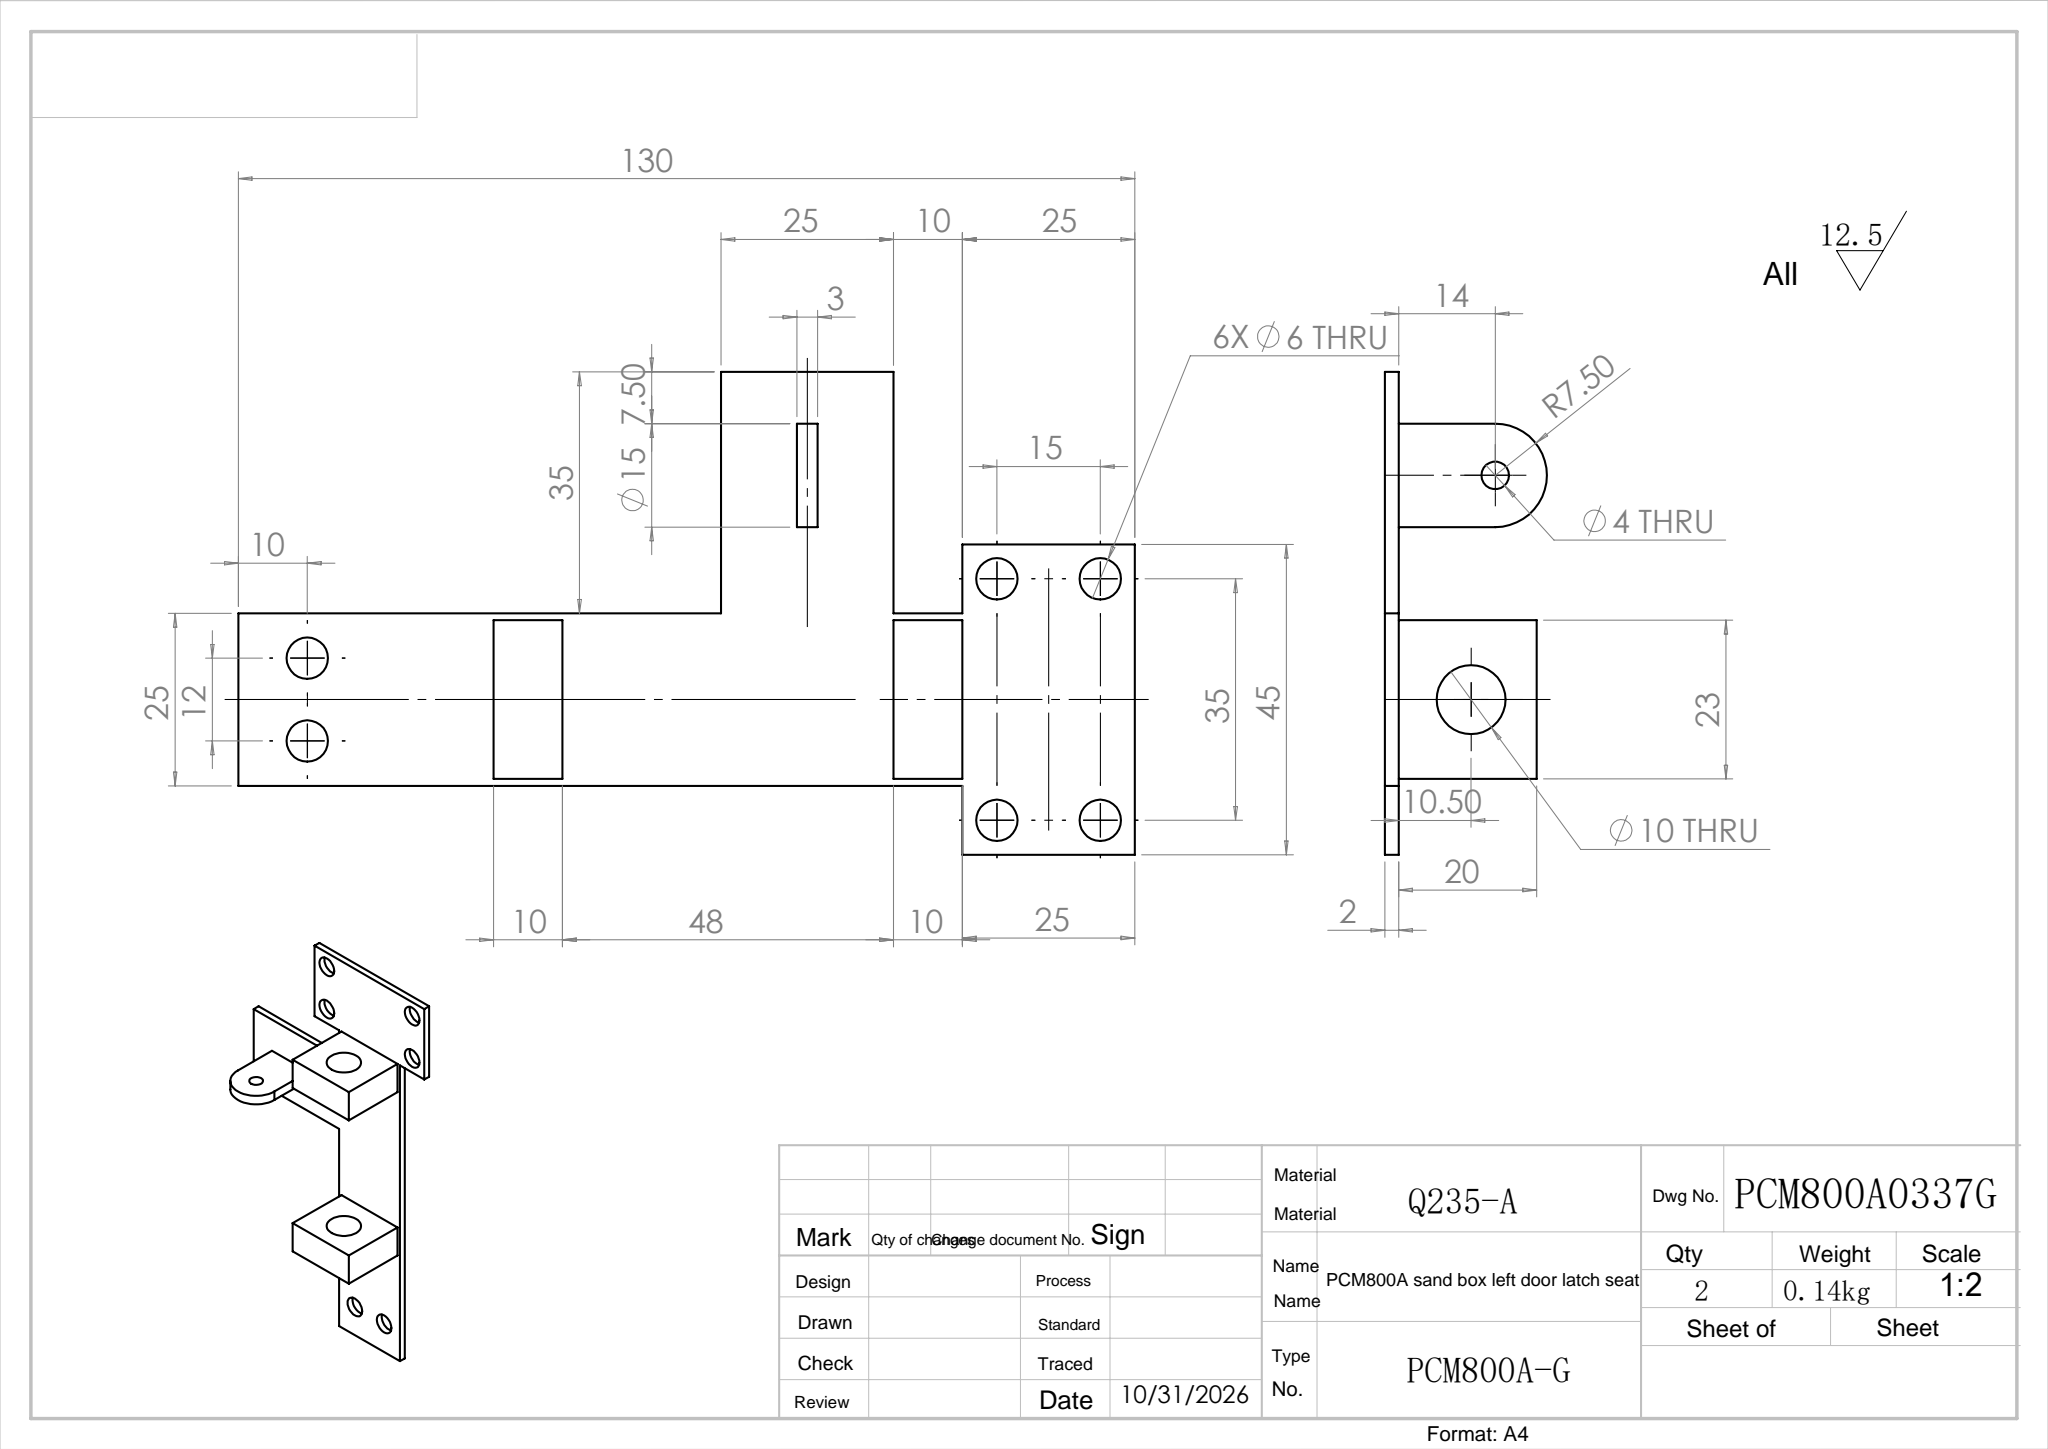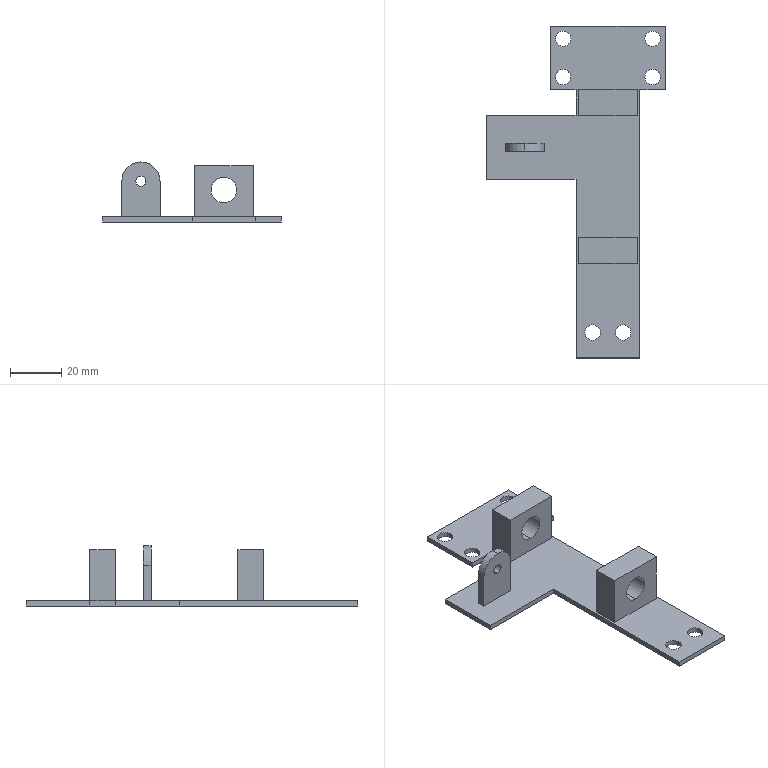Part | SolidWorks | features ICE 2, Extrusion 1, LPattern 1 | 1 solid | 48 faces | box 70 x 130 x 23.5 mm | volume 17397 mm3 | plane 28 | cylinder 20 | commonest cylinder face diameters 6 x12 10 x4 4 x2 15 x2